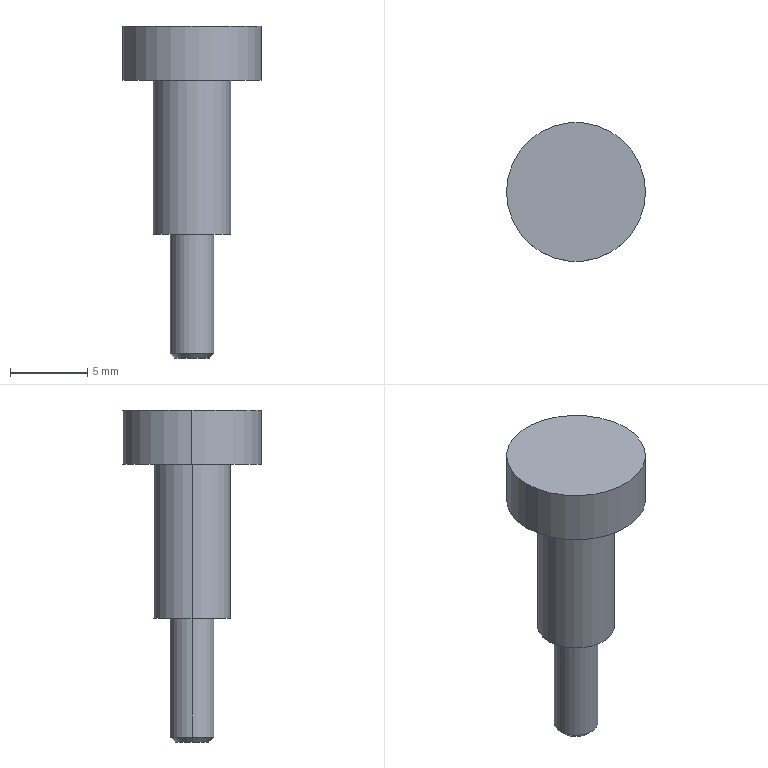Part | SolidWorks | features ICE 2, Extrusion 1, StudWizard 1 | 1 solid | 12 faces | box 9 x 9 x 21.5 mm | volume 469.445 mm3 | cylinder 6 | plane 4 | cone 2 | commonest cylinder face diameters 2.845 x2 5 x2 9 x2
STEP:
#1=CARTESIAN_POINT('',(1.106,0.,-21.5));
#2=VERTEX_POINT('',#1);
#3=CARTESIAN_POINT('',(-1.106,0.,-21.5));
#4=VERTEX_POINT('',#3);
#5=CARTESIAN_POINT('',(0.,0.,-21.5));
#6=DIRECTION('',(0.,0.,1.));
#7=DIRECTION('',(1.,0.,0.));
#8=AXIS2_PLACEMENT_3D('',#5,#6,#7);
#9=CIRCLE('',#8,1.106);
#10=EDGE_CURVE('',#2,#4,#9,.T.);
#11=ORIENTED_EDGE('',*,*,#10,.T.);
#12=CARTESIAN_POINT('',(-1.422,0.,-21.184));
#13=VERTEX_POINT('',#12);
#14=CARTESIAN_POINT('',(-1.106,0.,-21.5));
#15=DIRECTION('',(-0.7071,0.,0.7071));
#16=VECTOR('',#15,1000.);
#17=LINE('',#14,#16);
#18=EDGE_CURVE('',#4,#13,#17,.T.);
#19=ORIENTED_EDGE('',*,*,#18,.T.);
#20=CARTESIAN_POINT('',(1.422,0.,-21.184));
#21=VERTEX_POINT('',#20);
#22=CARTESIAN_POINT('',(0.,0.,-21.184));
#23=DIRECTION('',(0.,0.,1.));
#24=DIRECTION('',(1.,0.,0.));
#25=AXIS2_PLACEMENT_3D('',#22,#23,#24);
#26=CIRCLE('',#25,1.422);
#27=EDGE_CURVE('',#21,#13,#26,.T.);
#28=ORIENTED_EDGE('',*,*,#27,.F.);
#29=CARTESIAN_POINT('',(1.106,0.,-21.5));
#30=DIRECTION('',(0.7071,0.,0.7071));
#31=VECTOR('',#30,1000.);
#32=LINE('',#29,#31);
#33=EDGE_CURVE('',#2,#21,#32,.T.);
#34=ORIENTED_EDGE('',*,*,#33,.F.);
#35=EDGE_LOOP('',(#11,#19,#28,#34));
#36=FACE_OUTER_BOUND('',#35,.T.);
#37=CARTESIAN_POINT('',(0.,0.,-21.5));
#38=DIRECTION('',(0.,0.,1.));
#39=DIRECTION('',(1.,0.,0.));
#40=AXIS2_PLACEMENT_3D('',#37,#38,#39);
#41=CONICAL_SURFACE('',#40,1.106,0.7854);
#42=ADVANCED_FACE('',(#36),#41,.T.);
#43=ORIENTED_EDGE('',*,*,#27,.T.);
#44=CARTESIAN_POINT('',(-1.422,0.,-13.5));
#45=VERTEX_POINT('',#44);
#46=CARTESIAN_POINT('',(-1.422,0.,-21.5));
#47=DIRECTION('',(0.,0.,1.));
#48=VECTOR('',#47,1000.);
#49=LINE('',#46,#48);
#50=EDGE_CURVE('',#13,#45,#49,.T.);
#51=ORIENTED_EDGE('',*,*,#50,.T.);
#52=CARTESIAN_POINT('',(1.422,0.,-13.5));
#53=VERTEX_POINT('',#52);
#54=CARTESIAN_POINT('',(0.,0.,-13.5));
#55=DIRECTION('',(0.,0.,1.));
#56=DIRECTION('',(1.,0.,0.));
#57=AXIS2_PLACEMENT_3D('',#54,#55,#56);
#58=CIRCLE('',#57,1.422);
#59=EDGE_CURVE('',#53,#45,#58,.T.);
#60=ORIENTED_EDGE('',*,*,#59,.F.);
#61=CARTESIAN_POINT('',(1.422,0.,-21.5));
#62=DIRECTION('',(0.,0.,1.));
#63=VECTOR('',#62,1000.);
#64=LINE('',#61,#63);
#65=EDGE_CURVE('',#21,#53,#64,.T.);
#66=ORIENTED_EDGE('',*,*,#65,.F.);
#67=EDGE_LOOP('',(#43,#51,#60,#66));
#68=FACE_OUTER_BOUND('',#67,.T.);
#69=CARTESIAN_POINT('',(0.,0.,-21.5));
#70=DIRECTION('',(0.,0.,1.));
#71=DIRECTION('',(1.,0.,0.));
#72=AXIS2_PLACEMENT_3D('',#69,#70,#71);
#73=CYLINDRICAL_SURFACE('',#72,1.422);
#74=ADVANCED_FACE('',(#68),#73,.T.);
#75=CARTESIAN_POINT('',(-2.5,0.,-13.5));
#76=VERTEX_POINT('',#75);
#77=CARTESIAN_POINT('',(2.5,0.,-13.5));
#78=VERTEX_POINT('',#77);
#79=CARTESIAN_POINT('',(0.,0.,-13.5));
#80=DIRECTION('',(0.,0.,-1.));
#81=DIRECTION('',(-1.,0.,0.));
#82=AXIS2_PLACEMENT_3D('',#79,#80,#81);
#83=CIRCLE('',#82,2.5);
#84=EDGE_CURVE('',#76,#78,#83,.T.);
#85=ORIENTED_EDGE('',*,*,#84,.F.);
#86=CARTESIAN_POINT('',(-2.5,0.,-3.5));
#87=VERTEX_POINT('',#86);
#88=CARTESIAN_POINT('',(-2.5,0.,-13.5));
#89=DIRECTION('',(0.,0.,1.));
#90=VECTOR('',#89,1000.);
#91=LINE('',#88,#90);
#92=EDGE_CURVE('',#76,#87,#91,.T.);
#93=ORIENTED_EDGE('',*,*,#92,.T.);
#94=CARTESIAN_POINT('',(2.5,0.,-3.5));
#95=VERTEX_POINT('',#94);
#96=CARTESIAN_POINT('',(0.,0.,-3.5));
#97=DIRECTION('',(0.,0.,-1.));
#98=DIRECTION('',(-1.,0.,0.));
#99=AXIS2_PLACEMENT_3D('',#96,#97,#98);
#100=CIRCLE('',#99,2.5);
#101=EDGE_CURVE('',#87,#95,#100,.T.);
#102=ORIENTED_EDGE('',*,*,#101,.T.);
#103=CARTESIAN_POINT('',(2.5,0.,-13.5));
#104=DIRECTION('',(0.,0.,1.));
#105=VECTOR('',#104,1000.);
#106=LINE('',#103,#105);
#107=EDGE_CURVE('',#78,#95,#106,.T.);
#108=ORIENTED_EDGE('',*,*,#107,.F.);
#109=EDGE_LOOP('',(#85,#93,#102,#108));
#110=FACE_OUTER_BOUND('',#109,.T.);
#111=CARTESIAN_POINT('',(0.,0.,-13.5));
#112=DIRECTION('',(0.,0.,1.));
#113=DIRECTION('',(1.,0.,0.));
#114=AXIS2_PLACEMENT_3D('',#111,#112,#113);
#115=CYLINDRICAL_SURFACE('',#114,2.5);
#116=ADVANCED_FACE('',(#110),#115,.T.);
#117=CARTESIAN_POINT('',(4.5,0.,-3.5));
#118=VERTEX_POINT('',#117);
#119=CARTESIAN_POINT('',(-4.5,0.,-3.5));
#120=VERTEX_POINT('',#119);
#121=CARTESIAN_POINT('',(0.,0.,-3.5));
#122=DIRECTION('',(0.,0.,1.));
#123=DIRECTION('',(1.,0.,0.));
#124=AXIS2_PLACEMENT_3D('',#121,#122,#123);
#125=CIRCLE('',#124,4.5);
#126=EDGE_CURVE('',#118,#120,#125,.T.);
#127=ORIENTED_EDGE('',*,*,#126,.T.);
#128=CARTESIAN_POINT('',(-4.5,0.,0.));
#129=VERTEX_POINT('',#128);
#130=CARTESIAN_POINT('',(-4.5,0.,-3.5));
#131=DIRECTION('',(0.,0.,1.));
#132=VECTOR('',#131,1000.);
#133=LINE('',#130,#132);
#134=EDGE_CURVE('',#120,#129,#133,.T.);
#135=ORIENTED_EDGE('',*,*,#134,.T.);
#136=CARTESIAN_POINT('',(4.5,0.,0.));
#137=VERTEX_POINT('',#136);
#138=CARTESIAN_POINT('',(0.,0.,0.));
#139=DIRECTION('',(0.,0.,1.));
#140=DIRECTION('',(1.,0.,0.));
#141=AXIS2_PLACEMENT_3D('',#138,#139,#140);
#142=CIRCLE('',#141,4.5);
#143=EDGE_CURVE('',#137,#129,#142,.T.);
#144=ORIENTED_EDGE('',*,*,#143,.F.);
#145=CARTESIAN_POINT('',(4.5,0.,-3.5));
#146=DIRECTION('',(0.,0.,1.));
#147=VECTOR('',#146,1000.);
#148=LINE('',#145,#147);
#149=EDGE_CURVE('',#118,#137,#148,.T.);
#150=ORIENTED_EDGE('',*,*,#149,.F.);
#151=EDGE_LOOP('',(#127,#135,#144,#150));
#152=FACE_OUTER_BOUND('',#151,.T.);
#153=CARTESIAN_POINT('',(0.,0.,-3.5));
#154=DIRECTION('',(0.,0.,1.));
#155=DIRECTION('',(1.,0.,0.));
#156=AXIS2_PLACEMENT_3D('',#153,#154,#155);
#157=CYLINDRICAL_SURFACE('',#156,4.5);
#158=ADVANCED_FACE('',(#152),#157,.T.);
#159=ORIENTED_EDGE('',*,*,#134,.F.);
#160=CARTESIAN_POINT('',(0.,0.,-3.5));
#161=DIRECTION('',(0.,0.,1.));
#162=DIRECTION('',(1.,0.,0.));
#163=AXIS2_PLACEMENT_3D('',#160,#161,#162);
#164=CIRCLE('',#163,4.5);
#165=EDGE_CURVE('',#120,#118,#164,.T.);
#166=ORIENTED_EDGE('',*,*,#165,.T.);
#167=ORIENTED_EDGE('',*,*,#149,.T.);
#168=CARTESIAN_POINT('',(0.,0.,0.));
#169=DIRECTION('',(0.,0.,1.));
#170=DIRECTION('',(1.,0.,0.));
#171=AXIS2_PLACEMENT_3D('',#168,#169,#170);
#172=CIRCLE('',#171,4.5);
#173=EDGE_CURVE('',#129,#137,#172,.T.);
#174=ORIENTED_EDGE('',*,*,#173,.F.);
#175=EDGE_LOOP('',(#159,#166,#167,#174));
#176=FACE_OUTER_BOUND('',#175,.T.);
#177=CARTESIAN_POINT('',(0.,0.,-3.5));
#178=DIRECTION('',(0.,0.,1.));
#179=DIRECTION('',(1.,0.,0.));
#180=AXIS2_PLACEMENT_3D('',#177,#178,#179);
#181=CYLINDRICAL_SURFACE('',#180,4.5);
#182=ADVANCED_FACE('',(#176),#181,.T.);
#183=CARTESIAN_POINT('',(0.,0.,-3.5));
#184=DIRECTION('',(0.,0.,-1.));
#185=DIRECTION('',(-1.,0.,0.));
#186=AXIS2_PLACEMENT_3D('',#183,#184,#185);
#187=CIRCLE('',#186,2.5);
#188=EDGE_CURVE('',#95,#87,#187,.T.);
#189=ORIENTED_EDGE('',*,*,#188,.F.);
#190=ORIENTED_EDGE('',*,*,#101,.F.);
#191=EDGE_LOOP('',(#189,#190));
#192=FACE_BOUND('',#191,.T.);
#193=ORIENTED_EDGE('',*,*,#126,.F.);
#194=ORIENTED_EDGE('',*,*,#165,.F.);
#195=EDGE_LOOP('',(#193,#194));
#196=FACE_OUTER_BOUND('',#195,.T.);
#197=CARTESIAN_POINT('',(0.,0.,-3.5));
#198=DIRECTION('',(0.,0.,1.));
#199=DIRECTION('',(1.,0.,0.));
#200=AXIS2_PLACEMENT_3D('',#197,#198,#199);
#201=PLANE('',#200);
#202=ADVANCED_FACE('',(#192,#196),#201,.F.);
#203=ORIENTED_EDGE('',*,*,#143,.T.);
#204=ORIENTED_EDGE('',*,*,#173,.T.);
#205=EDGE_LOOP('',(#203,#204));
#206=FACE_OUTER_BOUND('',#205,.T.);
#207=CARTESIAN_POINT('',(0.,0.,0.));
#208=DIRECTION('',(0.,0.,1.));
#209=DIRECTION('',(1.,0.,0.));
#210=AXIS2_PLACEMENT_3D('',#207,#208,#209);
#211=PLANE('',#210);
#212=ADVANCED_FACE('',(#206),#211,.T.);
#213=ORIENTED_EDGE('',*,*,#92,.F.);
#214=CARTESIAN_POINT('',(0.,0.,-13.5));
#215=DIRECTION('',(0.,0.,-1.));
#216=DIRECTION('',(-1.,0.,0.));
#217=AXIS2_PLACEMENT_3D('',#214,#215,#216);
#218=CIRCLE('',#217,2.5);
#219=EDGE_CURVE('',#78,#76,#218,.T.);
#220=ORIENTED_EDGE('',*,*,#219,.F.);
#221=ORIENTED_EDGE('',*,*,#107,.T.);
#222=ORIENTED_EDGE('',*,*,#188,.T.);
#223=EDGE_LOOP('',(#213,#220,#221,#222));
#224=FACE_OUTER_BOUND('',#223,.T.);
#225=CARTESIAN_POINT('',(0.,0.,-13.5));
#226=DIRECTION('',(0.,0.,1.));
#227=DIRECTION('',(1.,0.,0.));
#228=AXIS2_PLACEMENT_3D('',#225,#226,#227);
#229=CYLINDRICAL_SURFACE('',#228,2.5);
#230=ADVANCED_FACE('',(#224),#229,.T.);
#231=ORIENTED_EDGE('',*,*,#219,.T.);
#232=ORIENTED_EDGE('',*,*,#84,.T.);
#233=EDGE_LOOP('',(#231,#232));
#234=FACE_OUTER_BOUND('',#233,.T.);
#235=ORIENTED_EDGE('',*,*,#59,.T.);
#236=CARTESIAN_POINT('',(0.,0.,-13.5));
#237=DIRECTION('',(0.,0.,1.));
#238=DIRECTION('',(1.,0.,0.));
#239=AXIS2_PLACEMENT_3D('',#236,#237,#238);
#240=CIRCLE('',#239,1.422);
#241=EDGE_CURVE('',#45,#53,#240,.T.);
#242=ORIENTED_EDGE('',*,*,#241,.T.);
#243=EDGE_LOOP('',(#235,#242));
#244=FACE_BOUND('',#243,.T.);
#245=CARTESIAN_POINT('',(0.,0.,-13.5));
#246=DIRECTION('',(0.,0.,-1.));
#247=DIRECTION('',(-1.,0.,0.));
#248=AXIS2_PLACEMENT_3D('',#245,#246,#247);
#249=PLANE('',#248);
#250=ADVANCED_FACE('',(#234,#244),#249,.T.);
#251=ORIENTED_EDGE('',*,*,#50,.F.);
#252=CARTESIAN_POINT('',(0.,0.,-21.184));
#253=DIRECTION('',(0.,0.,1.));
#254=DIRECTION('',(1.,0.,0.));
#255=AXIS2_PLACEMENT_3D('',#252,#253,#254);
#256=CIRCLE('',#255,1.422);
#257=EDGE_CURVE('',#13,#21,#256,.T.);
#258=ORIENTED_EDGE('',*,*,#257,.T.);
#259=ORIENTED_EDGE('',*,*,#65,.T.);
#260=ORIENTED_EDGE('',*,*,#241,.F.);
#261=EDGE_LOOP('',(#251,#258,#259,#260));
#262=FACE_OUTER_BOUND('',#261,.T.);
#263=CARTESIAN_POINT('',(0.,0.,-21.5));
#264=DIRECTION('',(0.,0.,1.));
#265=DIRECTION('',(1.,0.,0.));
#266=AXIS2_PLACEMENT_3D('',#263,#264,#265);
#267=CYLINDRICAL_SURFACE('',#266,1.422);
#268=ADVANCED_FACE('',(#262),#267,.T.);
#269=ORIENTED_EDGE('',*,*,#18,.F.);
#270=CARTESIAN_POINT('',(0.,0.,-21.5));
#271=DIRECTION('',(0.,0.,1.));
#272=DIRECTION('',(1.,0.,0.));
#273=AXIS2_PLACEMENT_3D('',#270,#271,#272);
#274=CIRCLE('',#273,1.106);
#275=EDGE_CURVE('',#4,#2,#274,.T.);
#276=ORIENTED_EDGE('',*,*,#275,.T.);
#277=ORIENTED_EDGE('',*,*,#33,.T.);
#278=ORIENTED_EDGE('',*,*,#257,.F.);
#279=EDGE_LOOP('',(#269,#276,#277,#278));
#280=FACE_OUTER_BOUND('',#279,.T.);
#281=CARTESIAN_POINT('',(0.,0.,-21.5));
#282=DIRECTION('',(0.,0.,1.));
#283=DIRECTION('',(1.,0.,0.));
#284=AXIS2_PLACEMENT_3D('',#281,#282,#283);
#285=CONICAL_SURFACE('',#284,1.106,0.7854);
#286=ADVANCED_FACE('',(#280),#285,.T.);
#287=ORIENTED_EDGE('',*,*,#10,.F.);
#288=ORIENTED_EDGE('',*,*,#275,.F.);
#289=EDGE_LOOP('',(#287,#288));
#290=FACE_OUTER_BOUND('',#289,.T.);
#291=CARTESIAN_POINT('',(0.,0.,-21.5));
#292=DIRECTION('',(0.,0.,-1.));
#293=DIRECTION('',(-1.,0.,0.));
#294=AXIS2_PLACEMENT_3D('',#291,#292,#293);
#295=PLANE('',#294);
#296=ADVANCED_FACE('',(#290),#295,.T.);
#297=CLOSED_SHELL('',(#42,#74,#116,#158,#182,#202,#212,#230,#250,#268,#286,#296));
#298=MANIFOLD_SOLID_BREP('',#297);
#299=CARTESIAN_POINT('',(0.,0.,0.));
#300=DIRECTION('',(0.,0.,1.));
#301=DIRECTION('',(1.,0.,0.));
#302=AXIS2_PLACEMENT_3D('',#299,#300,#301);
#303=(LENGTH_UNIT()NAMED_UNIT(*)SI_UNIT(.MILLI.,.METRE.));
#304=UNCERTAINTY_MEASURE_WITH_UNIT(LENGTH_MEASURE(0.00001),#303,'','');
#305=(NAMED_UNIT(*)PLANE_ANGLE_UNIT()SI_UNIT($,.RADIAN.));
#306=(NAMED_UNIT(*)SI_UNIT($,.STERADIAN.)SOLID_ANGLE_UNIT());
#307=(GEOMETRIC_REPRESENTATION_CONTEXT(3)GLOBAL_UNCERTAINTY_ASSIGNED_CONTEXT((#304))GLOBAL_UNIT_ASSIGNED_CONTEXT((#303,#305,#306))REPRESENTATION_CONTEXT('',''));
#308=ADVANCED_BREP_SHAPE_REPRESENTATION('',(#298,#302),#307);